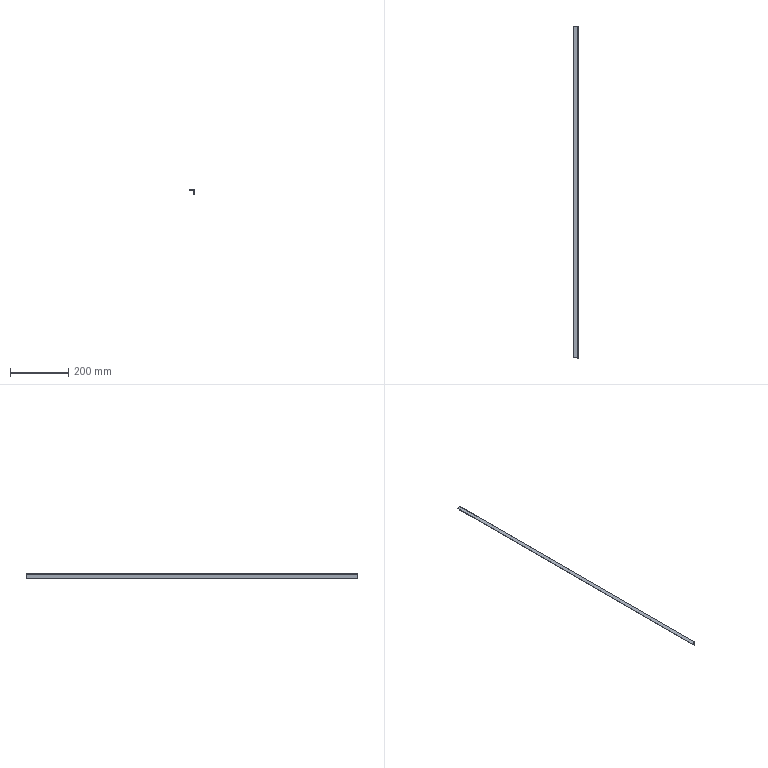Part | SolidWorks | features SplitBody 1 | 1 solid | 14 faces | box 15 x 1138 x 15 mm | volume 32695 mm3 | plane 12 | cylinder 2 | commonest cylinder face diameters 0.2 x1 2.2 x1
STEP:
#1=CARTESIAN_POINT('',(115.6,1258.5,298.8));
#2=VERTEX_POINT('',#1);
#3=CARTESIAN_POINT('',(115.6,1258.5,297.8));
#4=VERTEX_POINT('',#3);
#5=CARTESIAN_POINT('',(115.6,1258.5,298.8));
#6=DIRECTION('',(0.,0.,-1.));
#7=VECTOR('',#6,1000.);
#8=LINE('',#5,#7);
#9=EDGE_CURVE('',#2,#4,#8,.T.);
#10=ORIENTED_EDGE('',*,*,#9,.F.);
#11=CARTESIAN_POINT('',(116.7,1258.5,297.7));
#12=VERTEX_POINT('',#11);
#13=CARTESIAN_POINT('',(115.6,1258.5,297.7));
#14=DIRECTION('',(0.,-1.,0.));
#15=DIRECTION('',(-1.,0.,0.));
#16=AXIS2_PLACEMENT_3D('',#13,#14,#15);
#17=CIRCLE('',#16,1.1);
#18=EDGE_CURVE('',#12,#2,#17,.T.);
#19=ORIENTED_EDGE('',*,*,#18,.F.);
#20=CARTESIAN_POINT('',(115.7,1258.5,297.7));
#21=VERTEX_POINT('',#20);
#22=CARTESIAN_POINT('',(115.7,1258.5,297.7));
#23=DIRECTION('',(1.,0.,0.));
#24=VECTOR('',#23,1000.);
#25=LINE('',#22,#24);
#26=EDGE_CURVE('',#21,#12,#25,.T.);
#27=ORIENTED_EDGE('',*,*,#26,.F.);
#28=CARTESIAN_POINT('',(115.6,1258.5,297.7));
#29=DIRECTION('',(0.,-1.,0.));
#30=DIRECTION('',(1.,0.,0.));
#31=AXIS2_PLACEMENT_3D('',#28,#29,#30);
#32=CIRCLE('',#31,0.1);
#33=EDGE_CURVE('',#21,#4,#32,.T.);
#34=ORIENTED_EDGE('',*,*,#33,.T.);
#35=EDGE_LOOP('',(#10,#19,#27,#34));
#36=FACE_OUTER_BOUND('',#35,.T.);
#37=CARTESIAN_POINT('',(115.6,1258.5,298.8));
#38=DIRECTION('',(0.,1.,0.));
#39=DIRECTION('',(-1.,0.,0.));
#40=AXIS2_PLACEMENT_3D('',#37,#38,#39);
#41=PLANE('',#40);
#42=ADVANCED_FACE('',(#36),#41,.T.);
#43=CARTESIAN_POINT('',(101.7,1258.5,298.8));
#44=VERTEX_POINT('',#43);
#45=CARTESIAN_POINT('',(116.7,1258.5,298.8));
#46=DIRECTION('',(-1.,0.,0.));
#47=VECTOR('',#46,1000.);
#48=LINE('',#45,#47);
#49=EDGE_CURVE('',#2,#44,#48,.T.);
#50=ORIENTED_EDGE('',*,*,#49,.F.);
#51=ORIENTED_EDGE('',*,*,#9,.T.);
#52=CARTESIAN_POINT('',(101.7,1258.5,297.8));
#53=VERTEX_POINT('',#52);
#54=CARTESIAN_POINT('',(116.7,1258.5,297.8));
#55=DIRECTION('',(-1.,0.,0.));
#56=VECTOR('',#55,1000.);
#57=LINE('',#54,#56);
#58=EDGE_CURVE('',#4,#53,#57,.T.);
#59=ORIENTED_EDGE('',*,*,#58,.T.);
#60=CARTESIAN_POINT('',(101.7,1258.5,297.8));
#61=DIRECTION('',(0.,0.,1.));
#62=VECTOR('',#61,1000.);
#63=LINE('',#60,#62);
#64=EDGE_CURVE('',#53,#44,#63,.T.);
#65=ORIENTED_EDGE('',*,*,#64,.T.);
#66=EDGE_LOOP('',(#50,#51,#59,#65));
#67=FACE_OUTER_BOUND('',#66,.T.);
#68=CARTESIAN_POINT('',(115.7,1258.5,297.7));
#69=DIRECTION('',(0.,1.,0.));
#70=DIRECTION('',(-1.,0.,0.));
#71=AXIS2_PLACEMENT_3D('',#68,#69,#70);
#72=PLANE('',#71);
#73=ADVANCED_FACE('',(#67),#72,.T.);
#74=CARTESIAN_POINT('',(101.7,121.,298.8));
#75=VERTEX_POINT('',#74);
#76=CARTESIAN_POINT('',(115.6,121.,298.8));
#77=VERTEX_POINT('',#76);
#78=CARTESIAN_POINT('',(116.7,121.,298.8));
#79=DIRECTION('',(1.,0.,0.));
#80=VECTOR('',#79,1000.);
#81=LINE('',#78,#80);
#82=EDGE_CURVE('',#75,#77,#81,.T.);
#83=ORIENTED_EDGE('',*,*,#82,.T.);
#84=CARTESIAN_POINT('',(115.6,99.787,298.8));
#85=DIRECTION('',(0.,1.,0.));
#86=VECTOR('',#85,1000.);
#87=LINE('',#84,#86);
#88=EDGE_CURVE('',#77,#2,#87,.T.);
#89=ORIENTED_EDGE('',*,*,#88,.T.);
#90=ORIENTED_EDGE('',*,*,#49,.T.);
#91=CARTESIAN_POINT('',(101.7,99.787,298.8));
#92=DIRECTION('',(0.,1.,0.));
#93=VECTOR('',#92,1000.);
#94=LINE('',#91,#93);
#95=EDGE_CURVE('',#75,#44,#94,.T.);
#96=ORIENTED_EDGE('',*,*,#95,.F.);
#97=EDGE_LOOP('',(#83,#89,#90,#96));
#98=FACE_OUTER_BOUND('',#97,.T.);
#99=CARTESIAN_POINT('',(116.7,99.787,298.8));
#100=DIRECTION('',(0.,0.,-1.));
#101=DIRECTION('',(-1.,0.,0.));
#102=AXIS2_PLACEMENT_3D('',#99,#100,#101);
#103=PLANE('',#102);
#104=ADVANCED_FACE('',(#98),#103,.F.);
#105=CARTESIAN_POINT('',(101.7,121.,297.8));
#106=VERTEX_POINT('',#105);
#107=CARTESIAN_POINT('',(101.7,99.787,297.8));
#108=DIRECTION('',(0.,1.,0.));
#109=VECTOR('',#108,1000.);
#110=LINE('',#107,#109);
#111=EDGE_CURVE('',#106,#53,#110,.T.);
#112=ORIENTED_EDGE('',*,*,#111,.F.);
#113=CARTESIAN_POINT('',(101.7,121.,298.8));
#114=DIRECTION('',(0.,0.,-1.));
#115=VECTOR('',#114,1000.);
#116=LINE('',#113,#115);
#117=EDGE_CURVE('',#75,#106,#116,.T.);
#118=ORIENTED_EDGE('',*,*,#117,.F.);
#119=ORIENTED_EDGE('',*,*,#95,.T.);
#120=ORIENTED_EDGE('',*,*,#64,.F.);
#121=EDGE_LOOP('',(#112,#118,#119,#120));
#122=FACE_OUTER_BOUND('',#121,.T.);
#123=CARTESIAN_POINT('',(101.7,99.787,297.8));
#124=DIRECTION('',(-1.,0.,0.));
#125=DIRECTION('',(0.,-1.,0.));
#126=AXIS2_PLACEMENT_3D('',#123,#124,#125);
#127=PLANE('',#126);
#128=ADVANCED_FACE('',(#122),#127,.T.);
#129=CARTESIAN_POINT('',(115.6,121.,297.8));
#130=VERTEX_POINT('',#129);
#131=CARTESIAN_POINT('',(115.6,99.787,297.8));
#132=DIRECTION('',(0.,1.,0.));
#133=VECTOR('',#132,1000.);
#134=LINE('',#131,#133);
#135=EDGE_CURVE('',#130,#4,#134,.T.);
#136=ORIENTED_EDGE('',*,*,#135,.F.);
#137=CARTESIAN_POINT('',(116.7,121.,297.8));
#138=DIRECTION('',(1.,0.,0.));
#139=VECTOR('',#138,1000.);
#140=LINE('',#137,#139);
#141=EDGE_CURVE('',#106,#130,#140,.T.);
#142=ORIENTED_EDGE('',*,*,#141,.F.);
#143=ORIENTED_EDGE('',*,*,#111,.T.);
#144=ORIENTED_EDGE('',*,*,#58,.F.);
#145=EDGE_LOOP('',(#136,#142,#143,#144));
#146=FACE_OUTER_BOUND('',#145,.T.);
#147=CARTESIAN_POINT('',(116.7,99.787,297.8));
#148=DIRECTION('',(0.,0.,-1.));
#149=DIRECTION('',(-1.,0.,0.));
#150=AXIS2_PLACEMENT_3D('',#147,#148,#149);
#151=PLANE('',#150);
#152=ADVANCED_FACE('',(#146),#151,.T.);
#153=CARTESIAN_POINT('',(115.7,121.,297.7));
#154=VERTEX_POINT('',#153);
#155=CARTESIAN_POINT('',(115.7,99.787,297.7));
#156=DIRECTION('',(0.,1.,0.));
#157=VECTOR('',#156,1000.);
#158=LINE('',#155,#157);
#159=EDGE_CURVE('',#154,#21,#158,.T.);
#160=ORIENTED_EDGE('',*,*,#159,.F.);
#161=CARTESIAN_POINT('',(115.6,121.,297.7));
#162=DIRECTION('',(0.,1.,0.));
#163=DIRECTION('',(1.,0.,0.));
#164=AXIS2_PLACEMENT_3D('',#161,#162,#163);
#165=CIRCLE('',#164,0.1);
#166=EDGE_CURVE('',#130,#154,#165,.T.);
#167=ORIENTED_EDGE('',*,*,#166,.F.);
#168=ORIENTED_EDGE('',*,*,#135,.T.);
#169=ORIENTED_EDGE('',*,*,#33,.F.);
#170=EDGE_LOOP('',(#160,#167,#168,#169));
#171=FACE_OUTER_BOUND('',#170,.T.);
#172=CARTESIAN_POINT('',(115.6,99.787,297.7));
#173=DIRECTION('',(0.,1.,0.));
#174=DIRECTION('',(-1.,0.,0.));
#175=AXIS2_PLACEMENT_3D('',#172,#173,#174);
#176=CYLINDRICAL_SURFACE('',#175,0.1);
#177=ADVANCED_FACE('',(#171),#176,.F.);
#178=CARTESIAN_POINT('',(115.7,121.,283.8));
#179=VERTEX_POINT('',#178);
#180=CARTESIAN_POINT('',(115.7,1258.5,283.8));
#181=VERTEX_POINT('',#180);
#182=CARTESIAN_POINT('',(115.7,99.787,283.8));
#183=DIRECTION('',(0.,1.,0.));
#184=VECTOR('',#183,1000.);
#185=LINE('',#182,#184);
#186=EDGE_CURVE('',#179,#181,#185,.T.);
#187=ORIENTED_EDGE('',*,*,#186,.F.);
#188=CARTESIAN_POINT('',(115.7,121.,283.8));
#189=DIRECTION('',(0.,0.,-1.));
#190=VECTOR('',#189,1000.);
#191=LINE('',#188,#190);
#192=EDGE_CURVE('',#154,#179,#191,.T.);
#193=ORIENTED_EDGE('',*,*,#192,.F.);
#194=ORIENTED_EDGE('',*,*,#159,.T.);
#195=CARTESIAN_POINT('',(115.7,1258.5,283.8));
#196=DIRECTION('',(0.,0.,1.));
#197=VECTOR('',#196,1000.);
#198=LINE('',#195,#197);
#199=EDGE_CURVE('',#181,#21,#198,.T.);
#200=ORIENTED_EDGE('',*,*,#199,.F.);
#201=EDGE_LOOP('',(#187,#193,#194,#200));
#202=FACE_OUTER_BOUND('',#201,.T.);
#203=CARTESIAN_POINT('',(115.7,99.787,283.8));
#204=DIRECTION('',(-1.,0.,0.));
#205=DIRECTION('',(0.,-1.,0.));
#206=AXIS2_PLACEMENT_3D('',#203,#204,#205);
#207=PLANE('',#206);
#208=ADVANCED_FACE('',(#202),#207,.T.);
#209=CARTESIAN_POINT('',(116.7,121.,283.8));
#210=VERTEX_POINT('',#209);
#211=CARTESIAN_POINT('',(116.7,1258.5,283.8));
#212=VERTEX_POINT('',#211);
#213=CARTESIAN_POINT('',(116.7,99.787,283.8));
#214=DIRECTION('',(0.,1.,0.));
#215=VECTOR('',#214,1000.);
#216=LINE('',#213,#215);
#217=EDGE_CURVE('',#210,#212,#216,.T.);
#218=ORIENTED_EDGE('',*,*,#217,.F.);
#219=CARTESIAN_POINT('',(116.7,121.,283.8));
#220=DIRECTION('',(-1.,0.,0.));
#221=VECTOR('',#220,1000.);
#222=LINE('',#219,#221);
#223=EDGE_CURVE('',#210,#179,#222,.T.);
#224=ORIENTED_EDGE('',*,*,#223,.T.);
#225=ORIENTED_EDGE('',*,*,#186,.T.);
#226=CARTESIAN_POINT('',(116.7,1258.5,283.8));
#227=DIRECTION('',(-1.,0.,0.));
#228=VECTOR('',#227,1000.);
#229=LINE('',#226,#228);
#230=EDGE_CURVE('',#212,#181,#229,.T.);
#231=ORIENTED_EDGE('',*,*,#230,.F.);
#232=EDGE_LOOP('',(#218,#224,#225,#231));
#233=FACE_OUTER_BOUND('',#232,.T.);
#234=CARTESIAN_POINT('',(116.7,99.787,283.8));
#235=DIRECTION('',(0.,0.,-1.));
#236=DIRECTION('',(-1.,0.,0.));
#237=AXIS2_PLACEMENT_3D('',#234,#235,#236);
#238=PLANE('',#237);
#239=ADVANCED_FACE('',(#233),#238,.T.);
#240=CARTESIAN_POINT('',(116.7,121.,297.7));
#241=VERTEX_POINT('',#240);
#242=CARTESIAN_POINT('',(116.7,121.,283.8));
#243=DIRECTION('',(0.,0.,-1.));
#244=VECTOR('',#243,1000.);
#245=LINE('',#242,#244);
#246=EDGE_CURVE('',#241,#210,#245,.T.);
#247=ORIENTED_EDGE('',*,*,#246,.T.);
#248=ORIENTED_EDGE('',*,*,#217,.T.);
#249=CARTESIAN_POINT('',(116.7,1258.5,283.8));
#250=DIRECTION('',(0.,0.,1.));
#251=VECTOR('',#250,1000.);
#252=LINE('',#249,#251);
#253=EDGE_CURVE('',#212,#12,#252,.T.);
#254=ORIENTED_EDGE('',*,*,#253,.T.);
#255=CARTESIAN_POINT('',(116.7,99.787,297.7));
#256=DIRECTION('',(0.,1.,0.));
#257=VECTOR('',#256,1000.);
#258=LINE('',#255,#257);
#259=EDGE_CURVE('',#241,#12,#258,.T.);
#260=ORIENTED_EDGE('',*,*,#259,.F.);
#261=EDGE_LOOP('',(#247,#248,#254,#260));
#262=FACE_OUTER_BOUND('',#261,.T.);
#263=CARTESIAN_POINT('',(116.7,99.787,283.8));
#264=DIRECTION('',(-1.,0.,0.));
#265=DIRECTION('',(0.,-1.,0.));
#266=AXIS2_PLACEMENT_3D('',#263,#264,#265);
#267=PLANE('',#266);
#268=ADVANCED_FACE('',(#262),#267,.F.);
#269=CARTESIAN_POINT('',(115.6,121.,297.7));
#270=DIRECTION('',(0.,1.,0.));
#271=DIRECTION('',(-1.,0.,0.));
#272=AXIS2_PLACEMENT_3D('',#269,#270,#271);
#273=CIRCLE('',#272,1.1);
#274=EDGE_CURVE('',#77,#241,#273,.T.);
#275=ORIENTED_EDGE('',*,*,#274,.T.);
#276=ORIENTED_EDGE('',*,*,#259,.T.);
#277=ORIENTED_EDGE('',*,*,#18,.T.);
#278=ORIENTED_EDGE('',*,*,#88,.F.);
#279=EDGE_LOOP('',(#275,#276,#277,#278));
#280=FACE_OUTER_BOUND('',#279,.T.);
#281=CARTESIAN_POINT('',(115.6,99.787,297.7));
#282=DIRECTION('',(0.,1.,0.));
#283=DIRECTION('',(-1.,0.,0.));
#284=AXIS2_PLACEMENT_3D('',#281,#282,#283);
#285=CYLINDRICAL_SURFACE('',#284,1.1);
#286=ADVANCED_FACE('',(#280),#285,.T.);
#287=ORIENTED_EDGE('',*,*,#199,.T.);
#288=ORIENTED_EDGE('',*,*,#26,.T.);
#289=ORIENTED_EDGE('',*,*,#253,.F.);
#290=ORIENTED_EDGE('',*,*,#230,.T.);
#291=EDGE_LOOP('',(#287,#288,#289,#290));
#292=FACE_OUTER_BOUND('',#291,.T.);
#293=CARTESIAN_POINT('',(115.6,1258.5,297.7));
#294=DIRECTION('',(0.,-1.,0.));
#295=DIRECTION('',(1.,0.,0.));
#296=AXIS2_PLACEMENT_3D('',#293,#294,#295);
#297=PLANE('',#296);
#298=ADVANCED_FACE('',(#292),#297,.F.);
#299=CARTESIAN_POINT('',(115.6,121.,298.8));
#300=DIRECTION('',(0.,0.,-1.));
#301=VECTOR('',#300,1000.);
#302=LINE('',#299,#301);
#303=EDGE_CURVE('',#77,#130,#302,.T.);
#304=ORIENTED_EDGE('',*,*,#303,.F.);
#305=ORIENTED_EDGE('',*,*,#82,.F.);
#306=ORIENTED_EDGE('',*,*,#117,.T.);
#307=ORIENTED_EDGE('',*,*,#141,.T.);
#308=EDGE_LOOP('',(#304,#305,#306,#307));
#309=FACE_OUTER_BOUND('',#308,.T.);
#310=CARTESIAN_POINT('',(116.7,121.,298.8));
#311=DIRECTION('',(0.,1.,0.));
#312=DIRECTION('',(1.,0.,0.));
#313=AXIS2_PLACEMENT_3D('',#310,#311,#312);
#314=PLANE('',#313);
#315=ADVANCED_FACE('',(#309),#314,.F.);
#316=ORIENTED_EDGE('',*,*,#223,.F.);
#317=ORIENTED_EDGE('',*,*,#246,.F.);
#318=CARTESIAN_POINT('',(116.7,121.,297.7));
#319=DIRECTION('',(-1.,0.,0.));
#320=VECTOR('',#319,1000.);
#321=LINE('',#318,#320);
#322=EDGE_CURVE('',#241,#154,#321,.T.);
#323=ORIENTED_EDGE('',*,*,#322,.T.);
#324=ORIENTED_EDGE('',*,*,#192,.T.);
#325=EDGE_LOOP('',(#316,#317,#323,#324));
#326=FACE_OUTER_BOUND('',#325,.T.);
#327=CARTESIAN_POINT('',(116.7,121.,283.8));
#328=DIRECTION('',(0.,1.,0.));
#329=DIRECTION('',(0.,0.,-1.));
#330=AXIS2_PLACEMENT_3D('',#327,#328,#329);
#331=PLANE('',#330);
#332=ADVANCED_FACE('',(#326),#331,.F.);
#333=ORIENTED_EDGE('',*,*,#166,.T.);
#334=ORIENTED_EDGE('',*,*,#322,.F.);
#335=ORIENTED_EDGE('',*,*,#274,.F.);
#336=ORIENTED_EDGE('',*,*,#303,.T.);
#337=EDGE_LOOP('',(#333,#334,#335,#336));
#338=FACE_OUTER_BOUND('',#337,.T.);
#339=CARTESIAN_POINT('',(115.6,121.,297.7));
#340=DIRECTION('',(0.,-1.,0.));
#341=DIRECTION('',(1.,0.,0.));
#342=AXIS2_PLACEMENT_3D('',#339,#340,#341);
#343=PLANE('',#342);
#344=ADVANCED_FACE('',(#338),#343,.T.);
#345=CLOSED_SHELL('',(#42,#73,#104,#128,#152,#177,#208,#239,#268,#286,#298,#315,#332,#344));
#346=MANIFOLD_SOLID_BREP('',#345);
#347=CARTESIAN_POINT('',(0.,0.,0.));
#348=DIRECTION('',(0.,0.,1.));
#349=DIRECTION('',(1.,0.,0.));
#350=AXIS2_PLACEMENT_3D('',#347,#348,#349);
#351=(LENGTH_UNIT()NAMED_UNIT(*)SI_UNIT(.MILLI.,.METRE.));
#352=UNCERTAINTY_MEASURE_WITH_UNIT(LENGTH_MEASURE(0.00001),#351,'','');
#353=(NAMED_UNIT(*)PLANE_ANGLE_UNIT()SI_UNIT($,.RADIAN.));
#354=(NAMED_UNIT(*)SI_UNIT($,.STERADIAN.)SOLID_ANGLE_UNIT());
#355=(GEOMETRIC_REPRESENTATION_CONTEXT(3)GLOBAL_UNCERTAINTY_ASSIGNED_CONTEXT((#352))GLOBAL_UNIT_ASSIGNED_CONTEXT((#351,#353,#354))REPRESENTATION_CONTEXT('',''));
#356=ADVANCED_BREP_SHAPE_REPRESENTATION('',(#346,#350),#355);